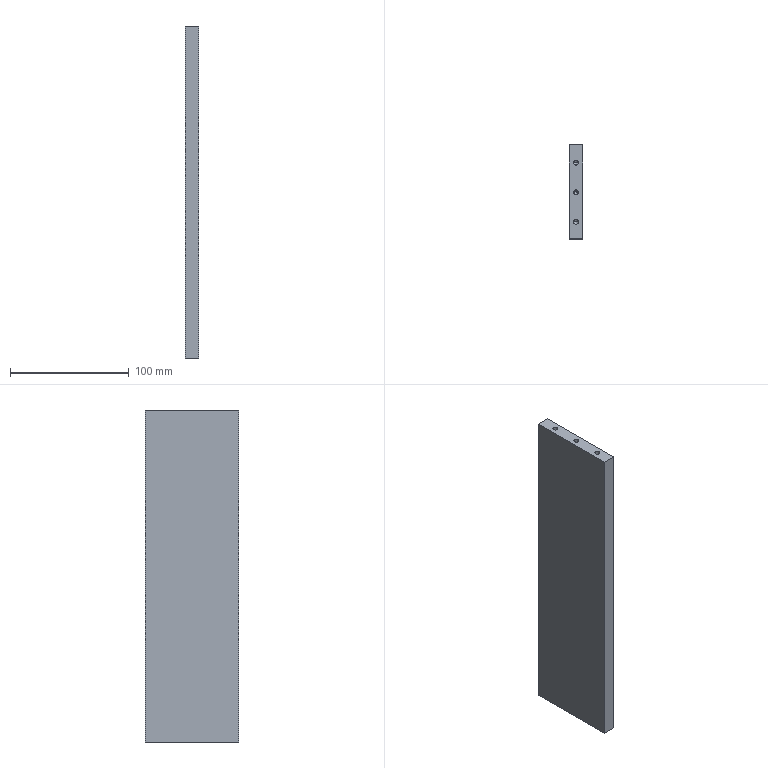Part | STEP file | PN_0070 (block) | 1 solid | 34 faces | box 11 x 79 x 280 mm | volume 242077 mm3 | cylinder 14 | cone 14 | plane 6 | commonest cylinder face diameters 4.2 x14